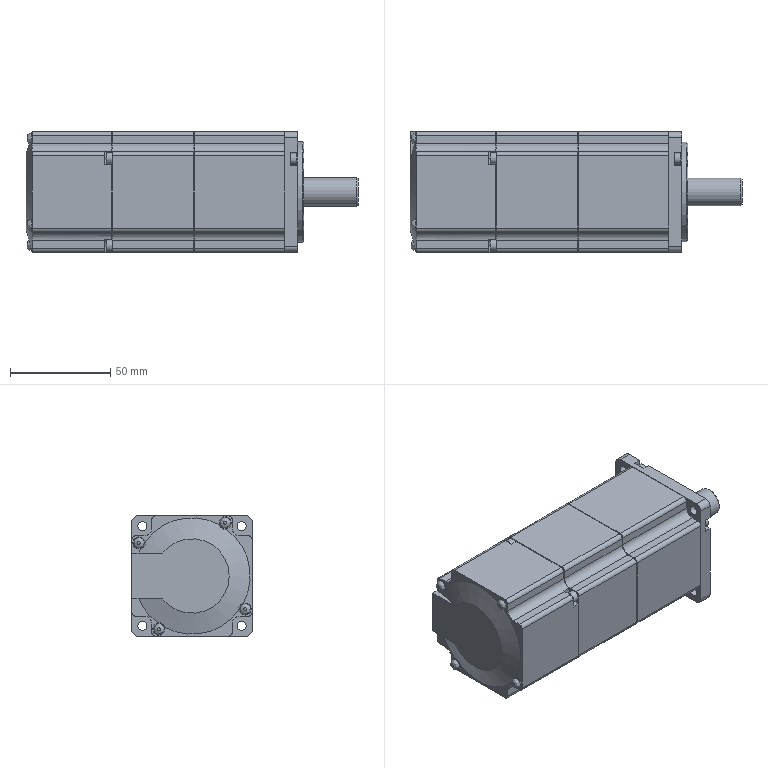Part | NX | 1 solid | 243 faces | box 165.5 x 60 x 60 mm | volume 440889 mm3 | plane 133 | cylinder 103 | spline 4 | cone 3 | commonest cylinder face diameters 4 x44 8 x24 6.5 x12 5.5 x8 6 x8 4.5 x4